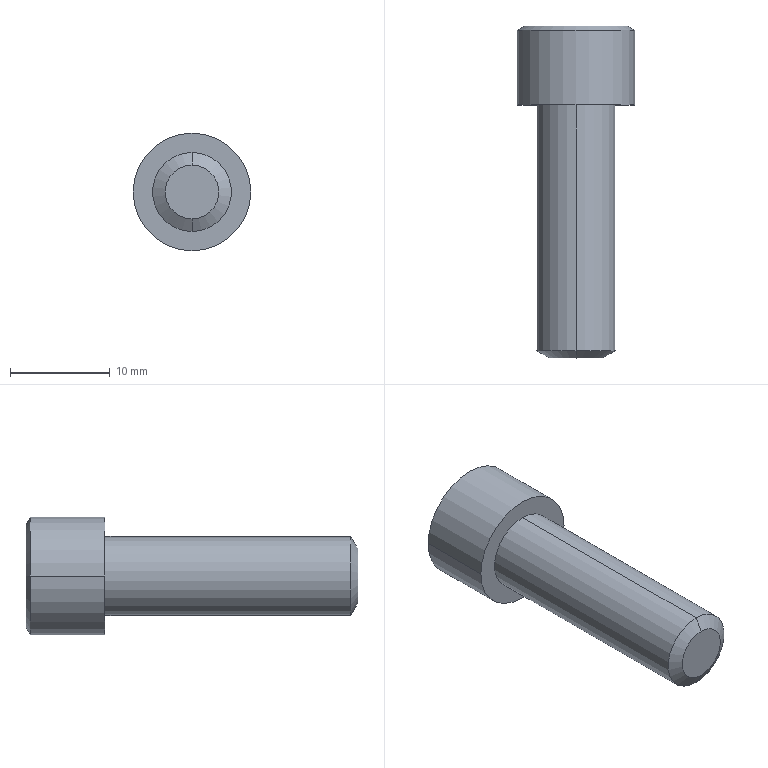Part | NX | features BREP 1 | 1 solid | 11 faces | box 11.811 x 33.325 x 11.811 mm | volume 2109 mm3 | cone 4 | cylinder 4 | plane 3 | commonest cylinder face diameters 7.938 x2 11.811 x2
STEP:
#1=CARTESIAN_POINT('',(0.,-25.4,2.699));
#2=VERTEX_POINT('',#1);
#3=CARTESIAN_POINT('',(0.,-25.4,-2.699));
#4=VERTEX_POINT('',#3);
#5=CARTESIAN_POINT('',(0.,-25.4,0.));
#6=DIRECTION('',(0.,-1.,0.));
#7=DIRECTION('',(0.,0.,1.));
#8=AXIS2_PLACEMENT_3D('',#5,#6,#7);
#9=CIRCLE('',#8,2.699);
#10=EDGE_CURVE('',#2,#4,#9,.T.);
#11=ORIENTED_EDGE('',*,*,#10,.T.);
#12=CARTESIAN_POINT('',(0.,-25.4,0.));
#13=DIRECTION('',(0.,-1.,0.));
#14=DIRECTION('',(0.,0.,-1.));
#15=AXIS2_PLACEMENT_3D('',#12,#13,#14);
#16=CIRCLE('',#15,2.699);
#17=EDGE_CURVE('',#4,#2,#16,.T.);
#18=ORIENTED_EDGE('',*,*,#17,.T.);
#19=EDGE_LOOP('',(#11,#18));
#20=FACE_BOUND('',#19,.T.);
#21=CARTESIAN_POINT('',(0.,-25.4,0.));
#22=DIRECTION('',(0.,-1.,0.));
#23=DIRECTION('',(0.,0.,-1.));
#24=AXIS2_PLACEMENT_3D('',#21,#22,#23);
#25=PLANE('',#24);
#26=ADVANCED_FACE('',(#20),#25,.T.);
#27=CARTESIAN_POINT('',(0.,-24.667,-3.969));
#28=VERTEX_POINT('',#27);
#29=CARTESIAN_POINT('',(0.,-25.4,-2.699));
#30=DIRECTION('',(0.,0.5,-0.866));
#31=VECTOR('',#30,1000.);
#32=LINE('',#29,#31);
#33=EDGE_CURVE('',#4,#28,#32,.T.);
#34=ORIENTED_EDGE('',*,*,#33,.T.);
#35=CARTESIAN_POINT('',(0.,-24.667,3.969));
#36=VERTEX_POINT('',#35);
#37=CARTESIAN_POINT('',(0.,-24.667,0.));
#38=DIRECTION('',(0.,-1.,0.));
#39=DIRECTION('',(0.,0.,-1.));
#40=AXIS2_PLACEMENT_3D('',#37,#38,#39);
#41=CIRCLE('',#40,3.969);
#42=EDGE_CURVE('',#28,#36,#41,.T.);
#43=ORIENTED_EDGE('',*,*,#42,.T.);
#44=CARTESIAN_POINT('',(0.,-25.4,2.699));
#45=DIRECTION('',(0.,0.5,0.866));
#46=VECTOR('',#45,1000.);
#47=LINE('',#44,#46);
#48=EDGE_CURVE('',#2,#36,#47,.T.);
#49=ORIENTED_EDGE('',*,*,#48,.F.);
#50=ORIENTED_EDGE('',*,*,#17,.F.);
#51=EDGE_LOOP('',(#34,#43,#49,#50));
#52=FACE_BOUND('',#51,.T.);
#53=CARTESIAN_POINT('',(0.,-25.033,0.));
#54=DIRECTION('',(0.,1.,0.));
#55=DIRECTION('',(0.,0.,1.));
#56=AXIS2_PLACEMENT_3D('',#53,#54,#55);
#57=CONICAL_SURFACE('',#56,3.334,1.047);
#58=ADVANCED_FACE('',(#52),#57,.T.);
#59=ORIENTED_EDGE('',*,*,#48,.T.);
#60=CARTESIAN_POINT('',(0.,-24.667,0.));
#61=DIRECTION('',(0.,-1.,0.));
#62=DIRECTION('',(0.,0.,1.));
#63=AXIS2_PLACEMENT_3D('',#60,#61,#62);
#64=CIRCLE('',#63,3.969);
#65=EDGE_CURVE('',#36,#28,#64,.T.);
#66=ORIENTED_EDGE('',*,*,#65,.T.);
#67=ORIENTED_EDGE('',*,*,#33,.F.);
#68=ORIENTED_EDGE('',*,*,#10,.F.);
#69=EDGE_LOOP('',(#59,#66,#67,#68));
#70=FACE_BOUND('',#69,.T.);
#71=CARTESIAN_POINT('',(0.,-25.033,0.));
#72=DIRECTION('',(0.,1.,0.));
#73=DIRECTION('',(0.,0.,1.));
#74=AXIS2_PLACEMENT_3D('',#71,#72,#73);
#75=CONICAL_SURFACE('',#74,3.334,1.047);
#76=ADVANCED_FACE('',(#70),#75,.T.);
#77=CARTESIAN_POINT('',(0.,0.,-3.969));
#78=VERTEX_POINT('',#77);
#79=CARTESIAN_POINT('',(0.,0.,-3.969));
#80=DIRECTION('',(0.,-1.,0.));
#81=VECTOR('',#80,1000.);
#82=LINE('',#79,#81);
#83=EDGE_CURVE('',#78,#28,#82,.T.);
#84=ORIENTED_EDGE('',*,*,#83,.T.);
#85=ORIENTED_EDGE('',*,*,#65,.F.);
#86=CARTESIAN_POINT('',(0.,0.,3.969));
#87=VERTEX_POINT('',#86);
#88=CARTESIAN_POINT('',(0.,0.,3.969));
#89=DIRECTION('',(0.,-1.,0.));
#90=VECTOR('',#89,1000.);
#91=LINE('',#88,#90);
#92=EDGE_CURVE('',#87,#36,#91,.T.);
#93=ORIENTED_EDGE('',*,*,#92,.F.);
#94=CARTESIAN_POINT('',(0.,0.,0.));
#95=DIRECTION('',(0.,-1.,0.));
#96=DIRECTION('',(0.,0.,1.));
#97=AXIS2_PLACEMENT_3D('',#94,#95,#96);
#98=CIRCLE('',#97,3.969);
#99=EDGE_CURVE('',#87,#78,#98,.T.);
#100=ORIENTED_EDGE('',*,*,#99,.T.);
#101=EDGE_LOOP('',(#84,#85,#93,#100));
#102=FACE_BOUND('',#101,.T.);
#103=CARTESIAN_POINT('',(0.,0.,0.));
#104=DIRECTION('',(0.,-1.,0.));
#105=DIRECTION('',(0.,0.,-1.));
#106=AXIS2_PLACEMENT_3D('',#103,#104,#105);
#107=CYLINDRICAL_SURFACE('',#106,3.969);
#108=ADVANCED_FACE('',(#102),#107,.T.);
#109=CARTESIAN_POINT('',(-5.905,0.,0.));
#110=VERTEX_POINT('',#109);
#111=CARTESIAN_POINT('',(5.905,0.,0.));
#112=VERTEX_POINT('',#111);
#113=CARTESIAN_POINT('',(0.,0.,0.));
#114=DIRECTION('',(0.,1.,0.));
#115=DIRECTION('',(-1.,0.,0.));
#116=AXIS2_PLACEMENT_3D('',#113,#114,#115);
#117=CIRCLE('',#116,5.905);
#118=EDGE_CURVE('',#110,#112,#117,.T.);
#119=ORIENTED_EDGE('',*,*,#118,.F.);
#120=CARTESIAN_POINT('',(0.,0.,0.));
#121=DIRECTION('',(0.,1.,0.));
#122=DIRECTION('',(1.,0.,0.));
#123=AXIS2_PLACEMENT_3D('',#120,#121,#122);
#124=CIRCLE('',#123,5.905);
#125=EDGE_CURVE('',#112,#110,#124,.T.);
#126=ORIENTED_EDGE('',*,*,#125,.F.);
#127=EDGE_LOOP('',(#119,#126));
#128=FACE_BOUND('',#127,.T.);
#129=ORIENTED_EDGE('',*,*,#99,.F.);
#130=CARTESIAN_POINT('',(0.,0.,0.));
#131=DIRECTION('',(0.,-1.,0.));
#132=DIRECTION('',(0.,0.,-1.));
#133=AXIS2_PLACEMENT_3D('',#130,#131,#132);
#134=CIRCLE('',#133,3.969);
#135=EDGE_CURVE('',#78,#87,#134,.T.);
#136=ORIENTED_EDGE('',*,*,#135,.F.);
#137=EDGE_LOOP('',(#129,#136));
#138=FACE_BOUND('',#137,.T.);
#139=CARTESIAN_POINT('',(0.,0.,0.));
#140=DIRECTION('',(0.,1.,0.));
#141=DIRECTION('',(1.,0.,0.));
#142=AXIS2_PLACEMENT_3D('',#139,#140,#141);
#143=PLANE('',#142);
#144=ADVANCED_FACE('',(#128,#138),#143,.F.);
#145=CARTESIAN_POINT('',(-5.905,7.485,0.));
#146=VERTEX_POINT('',#145);
#147=CARTESIAN_POINT('',(-5.905,0.,0.));
#148=DIRECTION('',(0.,1.,0.));
#149=VECTOR('',#148,1000.);
#150=LINE('',#147,#149);
#151=EDGE_CURVE('',#110,#146,#150,.T.);
#152=ORIENTED_EDGE('',*,*,#151,.T.);
#153=CARTESIAN_POINT('',(5.905,7.485,0.));
#154=VERTEX_POINT('',#153);
#155=CARTESIAN_POINT('',(0.,7.485,0.));
#156=DIRECTION('',(0.,1.,0.));
#157=DIRECTION('',(1.,0.,0.));
#158=AXIS2_PLACEMENT_3D('',#155,#156,#157);
#159=CIRCLE('',#158,5.905);
#160=EDGE_CURVE('',#154,#146,#159,.T.);
#161=ORIENTED_EDGE('',*,*,#160,.F.);
#162=CARTESIAN_POINT('',(5.905,0.,0.));
#163=DIRECTION('',(0.,1.,0.));
#164=VECTOR('',#163,1000.);
#165=LINE('',#162,#164);
#166=EDGE_CURVE('',#112,#154,#165,.T.);
#167=ORIENTED_EDGE('',*,*,#166,.F.);
#168=ORIENTED_EDGE('',*,*,#125,.T.);
#169=EDGE_LOOP('',(#152,#161,#167,#168));
#170=FACE_BOUND('',#169,.T.);
#171=CARTESIAN_POINT('',(0.,0.,0.));
#172=DIRECTION('',(0.,1.,0.));
#173=DIRECTION('',(1.,0.,0.));
#174=AXIS2_PLACEMENT_3D('',#171,#172,#173);
#175=CYLINDRICAL_SURFACE('',#174,5.905);
#176=ADVANCED_FACE('',(#170),#175,.T.);
#177=ORIENTED_EDGE('',*,*,#166,.T.);
#178=CARTESIAN_POINT('',(0.,7.485,0.));
#179=DIRECTION('',(0.,1.,0.));
#180=DIRECTION('',(-1.,0.,0.));
#181=AXIS2_PLACEMENT_3D('',#178,#179,#180);
#182=CIRCLE('',#181,5.905);
#183=EDGE_CURVE('',#146,#154,#182,.T.);
#184=ORIENTED_EDGE('',*,*,#183,.F.);
#185=ORIENTED_EDGE('',*,*,#151,.F.);
#186=ORIENTED_EDGE('',*,*,#118,.T.);
#187=EDGE_LOOP('',(#177,#184,#185,#186));
#188=FACE_BOUND('',#187,.T.);
#189=CARTESIAN_POINT('',(0.,0.,0.));
#190=DIRECTION('',(0.,1.,0.));
#191=DIRECTION('',(1.,0.,0.));
#192=AXIS2_PLACEMENT_3D('',#189,#190,#191);
#193=CYLINDRICAL_SURFACE('',#192,5.905);
#194=ADVANCED_FACE('',(#188),#193,.T.);
#195=CARTESIAN_POINT('',(-5.144,7.925,0.));
#196=VERTEX_POINT('',#195);
#197=CARTESIAN_POINT('',(-5.144,7.925,0.));
#198=DIRECTION('',(-0.866,-0.5,0.));
#199=VECTOR('',#198,1000.);
#200=LINE('',#197,#199);
#201=EDGE_CURVE('',#196,#146,#200,.T.);
#202=ORIENTED_EDGE('',*,*,#201,.T.);
#203=ORIENTED_EDGE('',*,*,#183,.T.);
#204=CARTESIAN_POINT('',(5.144,7.925,0.));
#205=VERTEX_POINT('',#204);
#206=CARTESIAN_POINT('',(5.144,7.925,0.));
#207=DIRECTION('',(0.866,-0.5,0.));
#208=VECTOR('',#207,1000.);
#209=LINE('',#206,#208);
#210=EDGE_CURVE('',#205,#154,#209,.T.);
#211=ORIENTED_EDGE('',*,*,#210,.F.);
#212=CARTESIAN_POINT('',(0.,7.925,0.));
#213=DIRECTION('',(0.,1.,0.));
#214=DIRECTION('',(-1.,0.,0.));
#215=AXIS2_PLACEMENT_3D('',#212,#213,#214);
#216=CIRCLE('',#215,5.144);
#217=EDGE_CURVE('',#196,#205,#216,.T.);
#218=ORIENTED_EDGE('',*,*,#217,.F.);
#219=EDGE_LOOP('',(#202,#203,#211,#218));
#220=FACE_BOUND('',#219,.T.);
#221=CARTESIAN_POINT('',(0.,7.705,0.));
#222=DIRECTION('',(0.,-1.,0.));
#223=DIRECTION('',(-1.,0.,0.));
#224=AXIS2_PLACEMENT_3D('',#221,#222,#223);
#225=CONICAL_SURFACE('',#224,5.524,1.047);
#226=ADVANCED_FACE('',(#220),#225,.T.);
#227=ORIENTED_EDGE('',*,*,#217,.T.);
#228=CARTESIAN_POINT('',(0.,7.925,0.));
#229=DIRECTION('',(0.,1.,0.));
#230=DIRECTION('',(1.,0.,0.));
#231=AXIS2_PLACEMENT_3D('',#228,#229,#230);
#232=CIRCLE('',#231,5.144);
#233=EDGE_CURVE('',#205,#196,#232,.T.);
#234=ORIENTED_EDGE('',*,*,#233,.T.);
#235=EDGE_LOOP('',(#227,#234));
#236=FACE_BOUND('',#235,.T.);
#237=CARTESIAN_POINT('',(0.,7.925,0.));
#238=DIRECTION('',(0.,1.,0.));
#239=DIRECTION('',(1.,0.,0.));
#240=AXIS2_PLACEMENT_3D('',#237,#238,#239);
#241=PLANE('',#240);
#242=ADVANCED_FACE('',(#236),#241,.T.);
#243=ORIENTED_EDGE('',*,*,#210,.T.);
#244=ORIENTED_EDGE('',*,*,#160,.T.);
#245=ORIENTED_EDGE('',*,*,#201,.F.);
#246=ORIENTED_EDGE('',*,*,#233,.F.);
#247=EDGE_LOOP('',(#243,#244,#245,#246));
#248=FACE_BOUND('',#247,.T.);
#249=CARTESIAN_POINT('',(0.,7.705,0.));
#250=DIRECTION('',(0.,-1.,0.));
#251=DIRECTION('',(-1.,0.,0.));
#252=AXIS2_PLACEMENT_3D('',#249,#250,#251);
#253=CONICAL_SURFACE('',#252,5.524,1.047);
#254=ADVANCED_FACE('',(#248),#253,.T.);
#255=ORIENTED_EDGE('',*,*,#92,.T.);
#256=ORIENTED_EDGE('',*,*,#42,.F.);
#257=ORIENTED_EDGE('',*,*,#83,.F.);
#258=ORIENTED_EDGE('',*,*,#135,.T.);
#259=EDGE_LOOP('',(#255,#256,#257,#258));
#260=FACE_BOUND('',#259,.T.);
#261=CARTESIAN_POINT('',(0.,0.,0.));
#262=DIRECTION('',(0.,-1.,0.));
#263=DIRECTION('',(0.,0.,-1.));
#264=AXIS2_PLACEMENT_3D('',#261,#262,#263);
#265=CYLINDRICAL_SURFACE('',#264,3.969);
#266=ADVANCED_FACE('',(#260),#265,.T.);
#267=CLOSED_SHELL('',(#26,#58,#76,#108,#144,#176,#194,#226,#242,#254,#266));
#268=MANIFOLD_SOLID_BREP('',#267);
#269=(LENGTH_UNIT()NAMED_UNIT(*)SI_UNIT(.MILLI.,.METRE.));
#270=UNCERTAINTY_MEASURE_WITH_UNIT(LENGTH_MEASURE(0.00001),#269,'','');
#271=(NAMED_UNIT(*)PLANE_ANGLE_UNIT()SI_UNIT($,.RADIAN.));
#272=(NAMED_UNIT(*)SI_UNIT($,.STERADIAN.)SOLID_ANGLE_UNIT());
#273=(GEOMETRIC_REPRESENTATION_CONTEXT(3)GLOBAL_UNCERTAINTY_ASSIGNED_CONTEXT((#270))GLOBAL_UNIT_ASSIGNED_CONTEXT((#269,#271,#272))REPRESENTATION_CONTEXT('',''));
#274=ADVANCED_BREP_SHAPE_REPRESENTATION('',(#268),#273);